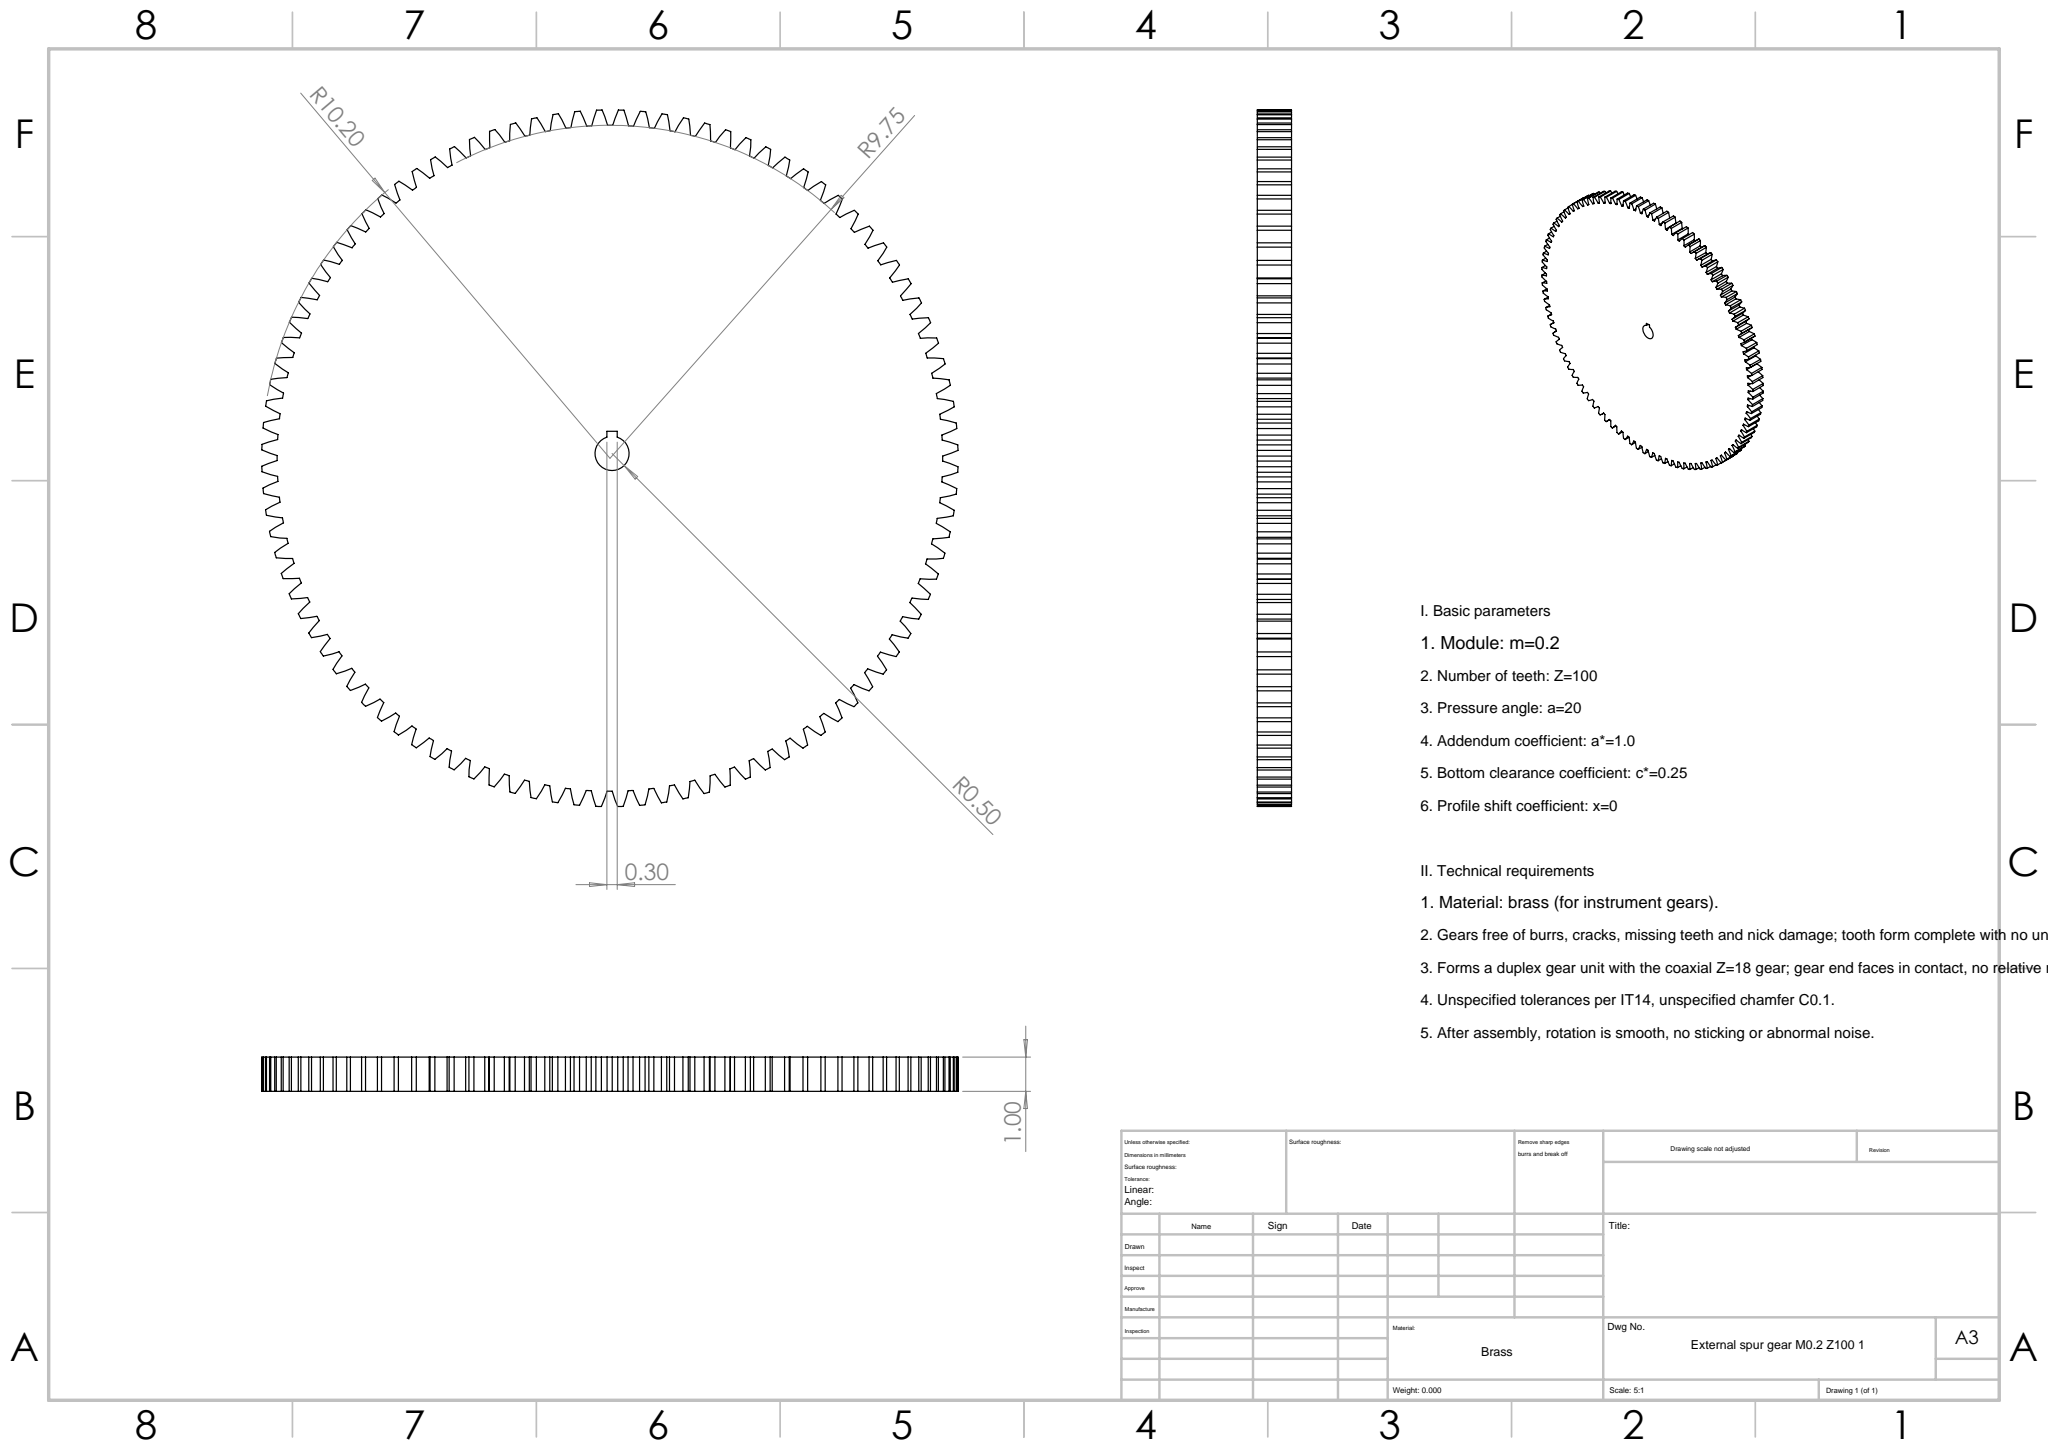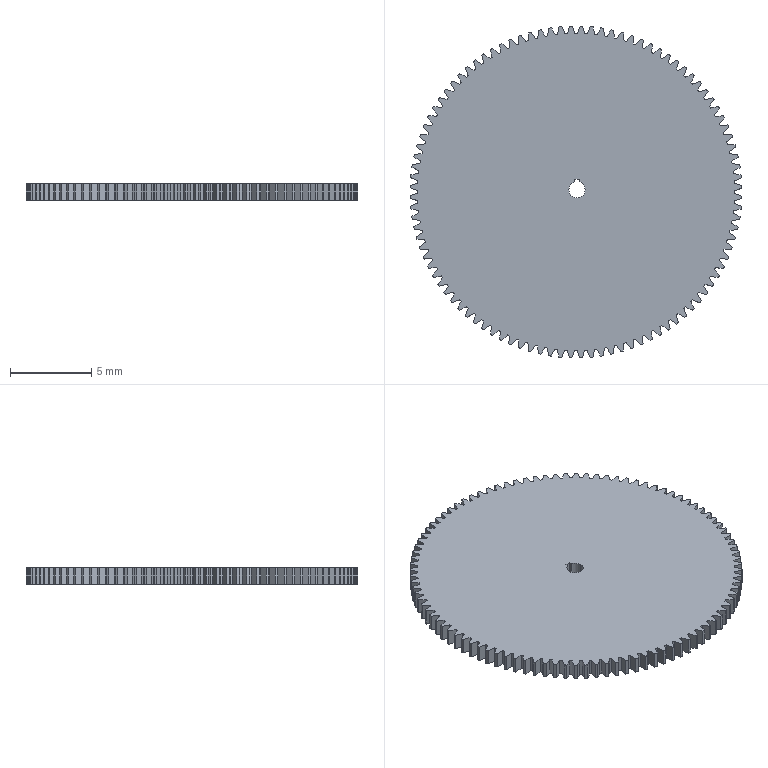Part | SolidWorks | features ICE 3, CirPattern 1, Extrusion 1 | 1 solid | 409 faces | box 20.395 x 20.395 x 1 mm | volume 312.456 mm3 | cylinder 204 | spline 200 | plane 5 | commonest cylinder face diameters 19.5 x101 20.4 x100 1 x3